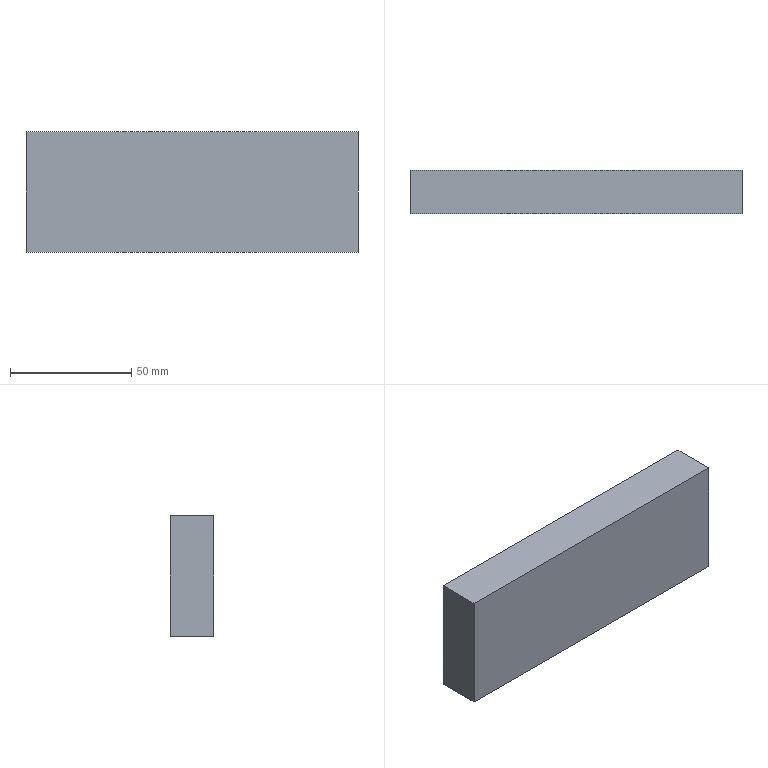Part | NX | 1 solid | 6 faces | box 137.023 x 18 x 49.799 mm | volume 122824 mm3 | plane 6
STEP:
#1=CARTESIAN_POINT('',(-187.326,-727.347,2435.287));
#2=VERTEX_POINT('',#1);
#3=CARTESIAN_POINT('',(-187.326,-727.347,2485.086));
#4=VERTEX_POINT('',#3);
#5=CARTESIAN_POINT('',(-187.326,-727.347,2435.287));
#6=DIRECTION('',(0.,0.,1.));
#7=VECTOR('',#6,1.);
#8=LINE('',#5,#7);
#9=EDGE_CURVE('',#2,#4,#8,.T.);
#10=ORIENTED_EDGE('',*,*,#9,.T.);
#11=CARTESIAN_POINT('',(-187.326,-709.347,2485.086));
#12=VERTEX_POINT('',#11);
#13=CARTESIAN_POINT('',(-187.326,-709.347,2485.086));
#14=DIRECTION('',(0.,-1.,0.));
#15=VECTOR('',#14,1.);
#16=LINE('',#13,#15);
#17=EDGE_CURVE('',#12,#4,#16,.T.);
#18=ORIENTED_EDGE('',*,*,#17,.F.);
#19=CARTESIAN_POINT('',(-187.326,-709.347,2435.287));
#20=VERTEX_POINT('',#19);
#21=CARTESIAN_POINT('',(-187.326,-709.347,2435.287));
#22=DIRECTION('',(0.,0.,1.));
#23=VECTOR('',#22,1.);
#24=LINE('',#21,#23);
#25=EDGE_CURVE('',#20,#12,#24,.T.);
#26=ORIENTED_EDGE('',*,*,#25,.F.);
#27=CARTESIAN_POINT('',(-187.326,-709.347,2435.287));
#28=DIRECTION('',(0.,-1.,0.));
#29=VECTOR('',#28,1.);
#30=LINE('',#27,#29);
#31=EDGE_CURVE('',#20,#2,#30,.T.);
#32=ORIENTED_EDGE('',*,*,#31,.T.);
#33=EDGE_LOOP('',(#10,#18,#26,#32));
#34=FACE_OUTER_BOUND('',#33,.T.);
#35=CARTESIAN_POINT('',(-187.326,-709.347,2435.287));
#36=DIRECTION('',(1.,0.,0.));
#37=DIRECTION('',(0.,0.,-1.));
#38=AXIS2_PLACEMENT_3D('',#35,#36,#37);
#39=PLANE('',#38);
#40=ADVANCED_FACE('',(#34),#39,.F.);
#41=CARTESIAN_POINT('',(-50.304,-727.347,2485.086));
#42=VERTEX_POINT('',#41);
#43=CARTESIAN_POINT('',(-187.326,-727.347,2485.086));
#44=DIRECTION('',(1.,0.,0.));
#45=VECTOR('',#44,1.);
#46=LINE('',#43,#45);
#47=EDGE_CURVE('',#4,#42,#46,.T.);
#48=ORIENTED_EDGE('',*,*,#47,.T.);
#49=CARTESIAN_POINT('',(-50.304,-709.347,2485.086));
#50=VERTEX_POINT('',#49);
#51=CARTESIAN_POINT('',(-50.304,-709.347,2485.086));
#52=DIRECTION('',(0.,-1.,0.));
#53=VECTOR('',#52,1.);
#54=LINE('',#51,#53);
#55=EDGE_CURVE('',#50,#42,#54,.T.);
#56=ORIENTED_EDGE('',*,*,#55,.F.);
#57=CARTESIAN_POINT('',(-187.326,-709.347,2485.086));
#58=DIRECTION('',(1.,0.,0.));
#59=VECTOR('',#58,1.);
#60=LINE('',#57,#59);
#61=EDGE_CURVE('',#12,#50,#60,.T.);
#62=ORIENTED_EDGE('',*,*,#61,.F.);
#63=ORIENTED_EDGE('',*,*,#17,.T.);
#64=EDGE_LOOP('',(#48,#56,#62,#63));
#65=FACE_OUTER_BOUND('',#64,.T.);
#66=CARTESIAN_POINT('',(-187.326,-709.347,2485.086));
#67=DIRECTION('',(0.,0.,-1.));
#68=DIRECTION('',(-1.,0.,0.));
#69=AXIS2_PLACEMENT_3D('',#66,#67,#68);
#70=PLANE('',#69);
#71=ADVANCED_FACE('',(#65),#70,.F.);
#72=CARTESIAN_POINT('',(-50.304,-727.347,2435.287));
#73=VERTEX_POINT('',#72);
#74=CARTESIAN_POINT('',(-50.304,-727.347,2435.287));
#75=DIRECTION('',(0.,0.,-1.));
#76=VECTOR('',#75,1.);
#77=LINE('',#74,#76);
#78=EDGE_CURVE('',#42,#73,#77,.T.);
#79=ORIENTED_EDGE('',*,*,#78,.T.);
#80=CARTESIAN_POINT('',(-50.304,-709.347,2435.287));
#81=VERTEX_POINT('',#80);
#82=CARTESIAN_POINT('',(-50.304,-709.347,2435.287));
#83=DIRECTION('',(0.,-1.,0.));
#84=VECTOR('',#83,1.);
#85=LINE('',#82,#84);
#86=EDGE_CURVE('',#81,#73,#85,.T.);
#87=ORIENTED_EDGE('',*,*,#86,.F.);
#88=CARTESIAN_POINT('',(-50.304,-709.347,2435.287));
#89=DIRECTION('',(0.,0.,-1.));
#90=VECTOR('',#89,1.);
#91=LINE('',#88,#90);
#92=EDGE_CURVE('',#50,#81,#91,.T.);
#93=ORIENTED_EDGE('',*,*,#92,.F.);
#94=ORIENTED_EDGE('',*,*,#55,.T.);
#95=EDGE_LOOP('',(#79,#87,#93,#94));
#96=FACE_OUTER_BOUND('',#95,.T.);
#97=CARTESIAN_POINT('',(-50.304,-709.347,2435.287));
#98=DIRECTION('',(-1.,0.,0.));
#99=DIRECTION('',(0.,0.,1.));
#100=AXIS2_PLACEMENT_3D('',#97,#98,#99);
#101=PLANE('',#100);
#102=ADVANCED_FACE('',(#96),#101,.F.);
#103=CARTESIAN_POINT('',(-187.326,-727.347,2435.287));
#104=DIRECTION('',(-1.,0.,0.));
#105=VECTOR('',#104,1.);
#106=LINE('',#103,#105);
#107=EDGE_CURVE('',#73,#2,#106,.T.);
#108=ORIENTED_EDGE('',*,*,#107,.T.);
#109=ORIENTED_EDGE('',*,*,#31,.F.);
#110=CARTESIAN_POINT('',(-187.326,-709.347,2435.287));
#111=DIRECTION('',(-1.,0.,0.));
#112=VECTOR('',#111,1.);
#113=LINE('',#110,#112);
#114=EDGE_CURVE('',#81,#20,#113,.T.);
#115=ORIENTED_EDGE('',*,*,#114,.F.);
#116=ORIENTED_EDGE('',*,*,#86,.T.);
#117=EDGE_LOOP('',(#108,#109,#115,#116));
#118=FACE_OUTER_BOUND('',#117,.T.);
#119=CARTESIAN_POINT('',(-187.326,-709.347,2435.287));
#120=DIRECTION('',(0.,0.,1.));
#121=DIRECTION('',(1.,0.,0.));
#122=AXIS2_PLACEMENT_3D('',#119,#120,#121);
#123=PLANE('',#122);
#124=ADVANCED_FACE('',(#118),#123,.F.);
#125=ORIENTED_EDGE('',*,*,#25,.T.);
#126=ORIENTED_EDGE('',*,*,#61,.T.);
#127=ORIENTED_EDGE('',*,*,#92,.T.);
#128=ORIENTED_EDGE('',*,*,#114,.T.);
#129=EDGE_LOOP('',(#125,#126,#127,#128));
#130=FACE_OUTER_BOUND('',#129,.T.);
#131=CARTESIAN_POINT('',(-187.326,-709.347,2485.086));
#132=DIRECTION('',(0.,1.,0.));
#133=DIRECTION('',(0.,0.,1.));
#134=AXIS2_PLACEMENT_3D('',#131,#132,#133);
#135=PLANE('',#134);
#136=ADVANCED_FACE('',(#130),#135,.T.);
#137=ORIENTED_EDGE('',*,*,#9,.F.);
#138=ORIENTED_EDGE('',*,*,#107,.F.);
#139=ORIENTED_EDGE('',*,*,#78,.F.);
#140=ORIENTED_EDGE('',*,*,#47,.F.);
#141=EDGE_LOOP('',(#137,#138,#139,#140));
#142=FACE_OUTER_BOUND('',#141,.T.);
#143=CARTESIAN_POINT('',(-187.326,-727.347,2485.086));
#144=DIRECTION('',(0.,1.,0.));
#145=DIRECTION('',(0.,0.,1.));
#146=AXIS2_PLACEMENT_3D('',#143,#144,#145);
#147=PLANE('',#146);
#148=ADVANCED_FACE('',(#142),#147,.F.);
#149=CLOSED_SHELL('',(#40,#71,#102,#124,#136,#148));
#150=MANIFOLD_SOLID_BREP('',#149);
#151=(LENGTH_UNIT()NAMED_UNIT(*)SI_UNIT(.MILLI.,.METRE.));
#152=UNCERTAINTY_MEASURE_WITH_UNIT(LENGTH_MEASURE(0.00002),#151,'','');
#153=(NAMED_UNIT(*)PLANE_ANGLE_UNIT()SI_UNIT($,.RADIAN.));
#154=PLANE_ANGLE_MEASURE_WITH_UNIT(PLANE_ANGLE_MEASURE(0.01745),#153);
#155=DIMENSIONAL_EXPONENTS(0.,0.,0.,0.,0.,0.,0.);
#156=(CONVERSION_BASED_UNIT('DEGREE',#154)NAMED_UNIT(#155)PLANE_ANGLE_UNIT());
#157=(NAMED_UNIT(*)SI_UNIT($,.STERADIAN.)SOLID_ANGLE_UNIT());
#158=(GEOMETRIC_REPRESENTATION_CONTEXT(3)GLOBAL_UNCERTAINTY_ASSIGNED_CONTEXT((#152))GLOBAL_UNIT_ASSIGNED_CONTEXT((#151,#156,#157))REPRESENTATION_CONTEXT('',''));
#159=ADVANCED_BREP_SHAPE_REPRESENTATION('',(#150),#158);